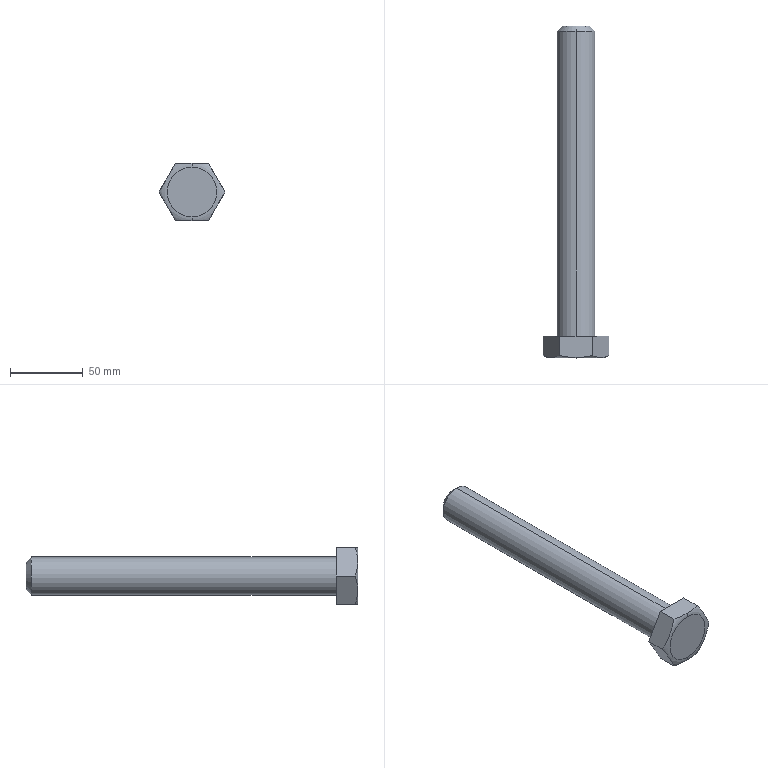Part | SolidWorks | features Chamfer 1, Extrusion 1, ICE 1, RevCut 1, Scale 1 | 1 solid | 15 faces | box 45.466 x 228.75 x 39.375 mm | volume 135169 mm3 | plane 9 | torus 2 | cone 2 | cylinder 2 | commonest cylinder face diameters 26.25 x2
STEP:
#1=CARTESIAN_POINT('',(11.367,-46.908,19.687));
#2=VERTEX_POINT('',#1);
#3=CARTESIAN_POINT('',(0.,-48.421,19.687));
#4=VERTEX_POINT('',#3);
#5=CARTESIAN_POINT('',(11.367,-46.908,19.687));
#6=CARTESIAN_POINT('',(10.465,-47.246,19.687));
#7=CARTESIAN_POINT('',(9.542,-47.5,19.687));
#8=CARTESIAN_POINT('',(7.671,-47.896,19.687));
#9=CARTESIAN_POINT('',(6.72,-48.038,19.687));
#10=CARTESIAN_POINT('',(4.805,-48.248,19.687));
#11=CARTESIAN_POINT('',(3.846,-48.315,19.687));
#12=CARTESIAN_POINT('',(1.925,-48.402,19.687));
#13=CARTESIAN_POINT('',(0.9641,-48.421,19.687));
#14=CARTESIAN_POINT('',(0.,-48.421,19.687));
#15=B_SPLINE_CURVE_WITH_KNOTS('',3,(#5,#6,#7,#8,#9,#10,#11,#12,#13,#14),.UNSPECIFIED.,.F.,.F.,(4,2,2,2,4),(0.07618,0.07906,0.08194,0.08482,0.08769),.UNSPECIFIED.);
#16=EDGE_CURVE('',#2,#4,#15,.T.);
#17=ORIENTED_EDGE('',*,*,#16,.T.);
#18=CARTESIAN_POINT('',(0.,-48.783,17.108));
#19=VERTEX_POINT('',#18);
#20=CARTESIAN_POINT('',(0.,-39.408,17.108));
#21=DIRECTION('',(1.,0.,0.));
#22=DIRECTION('',(0.,0.,-1.));
#23=AXIS2_PLACEMENT_3D('',#20,#21,#22);
#24=CIRCLE('',#23,9.375);
#25=EDGE_CURVE('',#4,#19,#24,.T.);
#26=ORIENTED_EDGE('',*,*,#25,.T.);
#27=CARTESIAN_POINT('',(0.,-48.783,-17.108));
#28=VERTEX_POINT('',#27);
#29=CARTESIAN_POINT('',(0.,-48.783,0.));
#30=DIRECTION('',(0.,-1.,0.));
#31=DIRECTION('',(0.,0.,-1.));
#32=AXIS2_PLACEMENT_3D('',#29,#30,#31);
#33=CIRCLE('',#32,17.108);
#34=EDGE_CURVE('',#28,#19,#33,.T.);
#35=ORIENTED_EDGE('',*,*,#34,.F.);
#36=CARTESIAN_POINT('',(0.,-48.421,-19.688));
#37=VERTEX_POINT('',#36);
#38=CARTESIAN_POINT('',(0.,-39.408,-17.108));
#39=DIRECTION('',(-1.,0.,0.));
#40=DIRECTION('',(0.,0.,1.));
#41=AXIS2_PLACEMENT_3D('',#38,#39,#40);
#42=CIRCLE('',#41,9.375);
#43=EDGE_CURVE('',#37,#28,#42,.T.);
#44=ORIENTED_EDGE('',*,*,#43,.F.);
#45=CARTESIAN_POINT('',(11.367,-46.908,-19.688));
#46=VERTEX_POINT('',#45);
#47=CARTESIAN_POINT('',(0.,-48.421,-19.688));
#48=CARTESIAN_POINT('',(0.9617,-48.421,-19.688));
#49=CARTESIAN_POINT('',(1.922,-48.402,-19.688));
#50=CARTESIAN_POINT('',(3.837,-48.315,-19.688));
#51=CARTESIAN_POINT('',(4.792,-48.248,-19.688));
#52=CARTESIAN_POINT('',(6.695,-48.041,-19.688));
#53=CARTESIAN_POINT('',(7.644,-47.901,-19.688));
#54=CARTESIAN_POINT('',(9.058,-47.603,-19.688));
#55=CARTESIAN_POINT('',(9.529,-47.488,-19.688));
#56=CARTESIAN_POINT('',(10.458,-47.226,-19.688));
#57=CARTESIAN_POINT('',(10.916,-47.077,-19.688));
#58=CARTESIAN_POINT('',(11.367,-46.908,-19.688));
#59=B_SPLINE_CURVE_WITH_KNOTS('',3,(#47,#48,#49,#50,#51,#52,#53,#54,#55,#56,#57,#58),.UNSPECIFIED.,.F.,.F.,(4,2,2,2,2,4),(0.,0.002872,0.005744,0.008616,0.01005,0.01149),.UNSPECIFIED.);
#60=EDGE_CURVE('',#37,#46,#59,.T.);
#61=ORIENTED_EDGE('',*,*,#60,.T.);
#62=CARTESIAN_POINT('',(22.733,-46.908,0.));
#63=VERTEX_POINT('',#62);
#64=CARTESIAN_POINT('',(11.367,-46.908,-19.688));
#65=CARTESIAN_POINT('',(11.821,-47.249,-18.901));
#66=CARTESIAN_POINT('',(12.283,-47.502,-18.1));
#67=CARTESIAN_POINT('',(13.219,-47.897,-16.479));
#68=CARTESIAN_POINT('',(13.693,-48.038,-15.659));
#69=CARTESIAN_POINT('',(14.646,-48.247,-14.007));
#70=CARTESIAN_POINT('',(15.128,-48.315,-13.173));
#71=CARTESIAN_POINT('',(16.087,-48.402,-11.511));
#72=CARTESIAN_POINT('',(16.567,-48.421,-10.681));
#73=CARTESIAN_POINT('',(17.524,-48.421,-9.022));
#74=CARTESIAN_POINT('',(18.003,-48.402,-8.193));
#75=CARTESIAN_POINT('',(18.959,-48.317,-6.537));
#76=CARTESIAN_POINT('',(19.437,-48.25,-5.709));
#77=CARTESIAN_POINT('',(20.152,-48.095,-4.47));
#78=CARTESIAN_POINT('',(20.391,-48.033,-4.057));
#79=CARTESIAN_POINT('',(20.867,-47.887,-3.233));
#80=CARTESIAN_POINT('',(21.105,-47.802,-2.82));
#81=CARTESIAN_POINT('',(21.814,-47.504,-1.591));
#82=CARTESIAN_POINT('',(22.28,-47.248,-0.7857));
#83=CARTESIAN_POINT('',(22.733,-46.908,0.));
#84=B_SPLINE_CURVE_WITH_KNOTS('',3,(#64,#65,#66,#67,#68,#69,#70,#71,#72,#73,#74,#75,#76,#77,#78,#79,#80,#81,#82,#83),.UNSPECIFIED.,.F.,.F.,(4,2,2,2,2,2,2,2,2,4),(0.000000456,0.00287,0.005739,0.008608,0.01148,0.01435,0.01722,0.01865,0.02008,0.02295),.UNSPECIFIED.);
#85=EDGE_CURVE('',#46,#63,#84,.T.);
#86=ORIENTED_EDGE('',*,*,#85,.T.);
#87=CARTESIAN_POINT('',(22.733,-46.908,0.));
#88=CARTESIAN_POINT('',(22.279,-47.249,0.7866));
#89=CARTESIAN_POINT('',(21.816,-47.502,1.588));
#90=CARTESIAN_POINT('',(20.881,-47.897,3.209));
#91=CARTESIAN_POINT('',(20.407,-48.038,4.029));
#92=CARTESIAN_POINT('',(19.453,-48.247,5.681));
#93=CARTESIAN_POINT('',(18.972,-48.315,6.514));
#94=CARTESIAN_POINT('',(18.013,-48.402,8.176));
#95=CARTESIAN_POINT('',(17.533,-48.421,9.007));
#96=CARTESIAN_POINT('',(16.575,-48.421,10.666));
#97=CARTESIAN_POINT('',(16.097,-48.402,11.495));
#98=CARTESIAN_POINT('',(15.14,-48.317,13.151));
#99=CARTESIAN_POINT('',(14.663,-48.25,13.978));
#100=CARTESIAN_POINT('',(13.947,-48.095,15.217));
#101=CARTESIAN_POINT('',(13.709,-48.033,15.63));
#102=CARTESIAN_POINT('',(13.233,-47.887,16.455));
#103=CARTESIAN_POINT('',(12.995,-47.802,16.868));
#104=CARTESIAN_POINT('',(12.285,-47.504,18.096));
#105=CARTESIAN_POINT('',(11.82,-47.248,18.902));
#106=CARTESIAN_POINT('',(11.367,-46.908,19.687));
#107=B_SPLINE_CURVE_WITH_KNOTS('',3,(#87,#88,#89,#90,#91,#92,#93,#94,#95,#96,#97,#98,#99,#100,#101,#102,#103,#104,#105,#106),.UNSPECIFIED.,.F.,.F.,(4,2,2,2,2,2,2,2,2,4),(0.000000456,0.00287,0.005739,0.008608,0.01148,0.01435,0.01722,0.01865,0.02008,0.02295),.UNSPECIFIED.);
#108=EDGE_CURVE('',#63,#2,#107,.T.);
#109=ORIENTED_EDGE('',*,*,#108,.T.);
#110=EDGE_LOOP('',(#17,#26,#35,#44,#61,#86,#109));
#111=FACE_OUTER_BOUND('',#110,.T.);
#112=CARTESIAN_POINT('',(0.,-39.408,0.));
#113=DIRECTION('',(0.,-1.,0.));
#114=DIRECTION('',(0.,0.,-1.));
#115=AXIS2_PLACEMENT_3D('',#112,#113,#114);
#116=TOROIDAL_SURFACE('',#115,17.108,9.375);
#117=ADVANCED_FACE('',(#111),#116,.T.);
#118=CARTESIAN_POINT('',(0.,179.967,9.375));
#119=VERTEX_POINT('',#118);
#120=CARTESIAN_POINT('',(0.,179.967,-9.375));
#121=VERTEX_POINT('',#120);
#122=CARTESIAN_POINT('',(0.,179.967,0.));
#123=DIRECTION('',(0.,1.,0.));
#124=DIRECTION('',(0.,0.,1.));
#125=AXIS2_PLACEMENT_3D('',#122,#123,#124);
#126=CIRCLE('',#125,9.375);
#127=EDGE_CURVE('',#119,#121,#126,.T.);
#128=ORIENTED_EDGE('',*,*,#127,.F.);
#129=CARTESIAN_POINT('',(0.,176.217,13.125));
#130=VERTEX_POINT('',#129);
#131=CARTESIAN_POINT('',(0.,179.967,9.375));
#132=DIRECTION('',(0.,-0.7071,0.7071));
#133=VECTOR('',#132,1000.);
#134=LINE('',#131,#133);
#135=EDGE_CURVE('',#119,#130,#134,.T.);
#136=ORIENTED_EDGE('',*,*,#135,.T.);
#137=CARTESIAN_POINT('',(0.,176.217,-13.125));
#138=VERTEX_POINT('',#137);
#139=CARTESIAN_POINT('',(0.,176.217,0.));
#140=DIRECTION('',(0.,-1.,0.));
#141=DIRECTION('',(0.,0.,1.));
#142=AXIS2_PLACEMENT_3D('',#139,#140,#141);
#143=CIRCLE('',#142,13.125);
#144=EDGE_CURVE('',#138,#130,#143,.T.);
#145=ORIENTED_EDGE('',*,*,#144,.F.);
#146=CARTESIAN_POINT('',(0.,179.967,-9.375));
#147=DIRECTION('',(0.,-0.7071,-0.7071));
#148=VECTOR('',#147,1000.);
#149=LINE('',#146,#148);
#150=EDGE_CURVE('',#121,#138,#149,.T.);
#151=ORIENTED_EDGE('',*,*,#150,.F.);
#152=EDGE_LOOP('',(#128,#136,#145,#151));
#153=FACE_OUTER_BOUND('',#152,.T.);
#154=CARTESIAN_POINT('',(0.,179.967,0.));
#155=DIRECTION('',(0.,-1.,0.));
#156=DIRECTION('',(0.,0.,-1.));
#157=AXIS2_PLACEMENT_3D('',#154,#155,#156);
#158=CONICAL_SURFACE('',#157,9.375,0.7854);
#159=ADVANCED_FACE('',(#153),#158,.T.);
#160=ORIENTED_EDGE('',*,*,#144,.T.);
#161=CARTESIAN_POINT('',(0.,-33.783,13.125));
#162=VERTEX_POINT('',#161);
#163=CARTESIAN_POINT('',(0.,179.967,13.125));
#164=DIRECTION('',(0.,-1.,0.));
#165=VECTOR('',#164,1000.);
#166=LINE('',#163,#165);
#167=EDGE_CURVE('',#130,#162,#166,.T.);
#168=ORIENTED_EDGE('',*,*,#167,.T.);
#169=CARTESIAN_POINT('',(0.,-33.783,-13.125));
#170=VERTEX_POINT('',#169);
#171=CARTESIAN_POINT('',(0.,-33.783,0.));
#172=DIRECTION('',(0.,1.,0.));
#173=DIRECTION('',(0.,0.,1.));
#174=AXIS2_PLACEMENT_3D('',#171,#172,#173);
#175=CIRCLE('',#174,13.125);
#176=EDGE_CURVE('',#162,#170,#175,.T.);
#177=ORIENTED_EDGE('',*,*,#176,.T.);
#178=CARTESIAN_POINT('',(0.,179.967,-13.125));
#179=DIRECTION('',(0.,-1.,0.));
#180=VECTOR('',#179,1000.);
#181=LINE('',#178,#180);
#182=EDGE_CURVE('',#138,#170,#181,.T.);
#183=ORIENTED_EDGE('',*,*,#182,.F.);
#184=EDGE_LOOP('',(#160,#168,#177,#183));
#185=FACE_OUTER_BOUND('',#184,.T.);
#186=CARTESIAN_POINT('',(0.,179.967,0.));
#187=DIRECTION('',(0.,-1.,0.));
#188=DIRECTION('',(0.,0.,-1.));
#189=AXIS2_PLACEMENT_3D('',#186,#187,#188);
#190=CYLINDRICAL_SURFACE('',#189,13.125);
#191=ADVANCED_FACE('',(#185),#190,.T.);
#192=ORIENTED_EDGE('',*,*,#108,.F.);
#193=CARTESIAN_POINT('',(22.733,-33.783,0.));
#194=VERTEX_POINT('',#193);
#195=CARTESIAN_POINT('',(22.733,-33.783,0.));
#196=DIRECTION('',(0.,-1.,0.));
#197=VECTOR('',#196,1000.);
#198=LINE('',#195,#197);
#199=EDGE_CURVE('',#194,#63,#198,.T.);
#200=ORIENTED_EDGE('',*,*,#199,.F.);
#201=CARTESIAN_POINT('',(11.367,-33.783,19.687));
#202=VERTEX_POINT('',#201);
#203=CARTESIAN_POINT('',(11.367,-33.783,19.687));
#204=DIRECTION('',(0.5,0.,-0.866));
#205=VECTOR('',#204,1000.);
#206=LINE('',#203,#205);
#207=EDGE_CURVE('',#202,#194,#206,.T.);
#208=ORIENTED_EDGE('',*,*,#207,.F.);
#209=CARTESIAN_POINT('',(11.367,-33.783,19.687));
#210=DIRECTION('',(0.,-1.,0.));
#211=VECTOR('',#210,1000.);
#212=LINE('',#209,#211);
#213=EDGE_CURVE('',#202,#2,#212,.T.);
#214=ORIENTED_EDGE('',*,*,#213,.T.);
#215=EDGE_LOOP('',(#192,#200,#208,#214));
#216=FACE_OUTER_BOUND('',#215,.T.);
#217=CARTESIAN_POINT('',(11.367,-33.783,19.687));
#218=DIRECTION('',(-0.866,0.,-0.5));
#219=DIRECTION('',(-0.5,0.,0.866));
#220=AXIS2_PLACEMENT_3D('',#217,#218,#219);
#221=PLANE('',#220);
#222=ADVANCED_FACE('',(#216),#221,.F.);
#223=ORIENTED_EDGE('',*,*,#85,.F.);
#224=CARTESIAN_POINT('',(11.367,-33.783,-19.688));
#225=VERTEX_POINT('',#224);
#226=CARTESIAN_POINT('',(11.367,-33.783,-19.688));
#227=DIRECTION('',(0.,-1.,0.));
#228=VECTOR('',#227,1000.);
#229=LINE('',#226,#228);
#230=EDGE_CURVE('',#225,#46,#229,.T.);
#231=ORIENTED_EDGE('',*,*,#230,.F.);
#232=CARTESIAN_POINT('',(22.733,-33.783,0.));
#233=DIRECTION('',(-0.5,0.,-0.866));
#234=VECTOR('',#233,1000.);
#235=LINE('',#232,#234);
#236=EDGE_CURVE('',#194,#225,#235,.T.);
#237=ORIENTED_EDGE('',*,*,#236,.F.);
#238=ORIENTED_EDGE('',*,*,#199,.T.);
#239=EDGE_LOOP('',(#223,#231,#237,#238));
#240=FACE_OUTER_BOUND('',#239,.T.);
#241=CARTESIAN_POINT('',(22.733,-33.783,0.));
#242=DIRECTION('',(-0.866,0.,0.5));
#243=DIRECTION('',(0.5,0.,0.866));
#244=AXIS2_PLACEMENT_3D('',#241,#242,#243);
#245=PLANE('',#244);
#246=ADVANCED_FACE('',(#240),#245,.F.);
#247=CARTESIAN_POINT('',(-11.367,-46.908,-19.688));
#248=VERTEX_POINT('',#247);
#249=CARTESIAN_POINT('',(-11.367,-46.908,-19.688));
#250=CARTESIAN_POINT('',(-10.465,-47.246,-19.688));
#251=CARTESIAN_POINT('',(-9.542,-47.5,-19.688));
#252=CARTESIAN_POINT('',(-7.671,-47.896,-19.687));
#253=CARTESIAN_POINT('',(-6.72,-48.038,-19.688));
#254=CARTESIAN_POINT('',(-4.805,-48.248,-19.688));
#255=CARTESIAN_POINT('',(-3.846,-48.315,-19.688));
#256=CARTESIAN_POINT('',(-1.925,-48.402,-19.688));
#257=CARTESIAN_POINT('',(-0.9641,-48.421,-19.688));
#258=CARTESIAN_POINT('',(0.,-48.421,-19.688));
#259=B_SPLINE_CURVE_WITH_KNOTS('',3,(#249,#250,#251,#252,#253,#254,#255,#256,#257,#258),.UNSPECIFIED.,.F.,.F.,(4,2,2,2,4),(0.07618,0.07906,0.08194,0.08482,0.08769),.UNSPECIFIED.);
#260=EDGE_CURVE('',#248,#37,#259,.T.);
#261=ORIENTED_EDGE('',*,*,#260,.F.);
#262=CARTESIAN_POINT('',(-11.367,-33.783,-19.688));
#263=VERTEX_POINT('',#262);
#264=CARTESIAN_POINT('',(-11.367,-33.783,-19.688));
#265=DIRECTION('',(0.,-1.,0.));
#266=VECTOR('',#265,1000.);
#267=LINE('',#264,#266);
#268=EDGE_CURVE('',#263,#248,#267,.T.);
#269=ORIENTED_EDGE('',*,*,#268,.F.);
#270=CARTESIAN_POINT('',(11.367,-33.783,-19.688));
#271=DIRECTION('',(-1.,0.,0.));
#272=VECTOR('',#271,1000.);
#273=LINE('',#270,#272);
#274=EDGE_CURVE('',#225,#263,#273,.T.);
#275=ORIENTED_EDGE('',*,*,#274,.F.);
#276=ORIENTED_EDGE('',*,*,#230,.T.);
#277=ORIENTED_EDGE('',*,*,#60,.F.);
#278=EDGE_LOOP('',(#261,#269,#275,#276,#277));
#279=FACE_OUTER_BOUND('',#278,.T.);
#280=CARTESIAN_POINT('',(11.367,-33.783,-19.688));
#281=DIRECTION('',(0.,0.,1.));
#282=DIRECTION('',(1.,0.,0.));
#283=AXIS2_PLACEMENT_3D('',#280,#281,#282);
#284=PLANE('',#283);
#285=ADVANCED_FACE('',(#279),#284,.F.);
#286=CARTESIAN_POINT('',(-22.733,-46.908,0.));
#287=VERTEX_POINT('',#286);
#288=CARTESIAN_POINT('',(-22.733,-46.908,0.));
#289=CARTESIAN_POINT('',(-22.279,-47.249,-0.7866));
#290=CARTESIAN_POINT('',(-21.816,-47.502,-1.588));
#291=CARTESIAN_POINT('',(-20.881,-47.897,-3.209));
#292=CARTESIAN_POINT('',(-20.407,-48.038,-4.029));
#293=CARTESIAN_POINT('',(-19.453,-48.247,-5.681));
#294=CARTESIAN_POINT('',(-18.972,-48.315,-6.514));
#295=CARTESIAN_POINT('',(-18.013,-48.402,-8.176));
#296=CARTESIAN_POINT('',(-17.533,-48.421,-9.007));
#297=CARTESIAN_POINT('',(-16.575,-48.421,-10.666));
#298=CARTESIAN_POINT('',(-16.097,-48.402,-11.495));
#299=CARTESIAN_POINT('',(-15.14,-48.317,-13.151));
#300=CARTESIAN_POINT('',(-14.663,-48.25,-13.978));
#301=CARTESIAN_POINT('',(-13.947,-48.095,-15.217));
#302=CARTESIAN_POINT('',(-13.709,-48.033,-15.63));
#303=CARTESIAN_POINT('',(-13.233,-47.887,-16.455));
#304=CARTESIAN_POINT('',(-12.995,-47.802,-16.868));
#305=CARTESIAN_POINT('',(-12.285,-47.504,-18.096));
#306=CARTESIAN_POINT('',(-11.82,-47.248,-18.902));
#307=CARTESIAN_POINT('',(-11.367,-46.908,-19.688));
#308=B_SPLINE_CURVE_WITH_KNOTS('',3,(#288,#289,#290,#291,#292,#293,#294,#295,#296,#297,#298,#299,#300,#301,#302,#303,#304,#305,#306,#307),.UNSPECIFIED.,.F.,.F.,(4,2,2,2,2,2,2,2,2,4),(0.000000456,0.00287,0.005739,0.008608,0.01148,0.01435,0.01722,0.01865,0.02008,0.02295),.UNSPECIFIED.);
#309=EDGE_CURVE('',#287,#248,#308,.T.);
#310=ORIENTED_EDGE('',*,*,#309,.F.);
#311=CARTESIAN_POINT('',(-22.733,-33.783,0.));
#312=VERTEX_POINT('',#311);
#313=CARTESIAN_POINT('',(-22.733,-33.783,0.));
#314=DIRECTION('',(0.,-1.,0.));
#315=VECTOR('',#314,1000.);
#316=LINE('',#313,#315);
#317=EDGE_CURVE('',#312,#287,#316,.T.);
#318=ORIENTED_EDGE('',*,*,#317,.F.);
#319=CARTESIAN_POINT('',(-11.367,-33.783,-19.688));
#320=DIRECTION('',(-0.5,0.,0.866));
#321=VECTOR('',#320,1000.);
#322=LINE('',#319,#321);
#323=EDGE_CURVE('',#263,#312,#322,.T.);
#324=ORIENTED_EDGE('',*,*,#323,.F.);
#325=ORIENTED_EDGE('',*,*,#268,.T.);
#326=EDGE_LOOP('',(#310,#318,#324,#325));
#327=FACE_OUTER_BOUND('',#326,.T.);
#328=CARTESIAN_POINT('',(-11.367,-33.783,-19.688));
#329=DIRECTION('',(0.866,0.,0.5));
#330=DIRECTION('',(0.5,0.,-0.866));
#331=AXIS2_PLACEMENT_3D('',#328,#329,#330);
#332=PLANE('',#331);
#333=ADVANCED_FACE('',(#327),#332,.F.);
#334=CARTESIAN_POINT('',(-11.367,-46.908,19.687));
#335=VERTEX_POINT('',#334);
#336=CARTESIAN_POINT('',(-11.367,-46.908,19.687));
#337=CARTESIAN_POINT('',(-11.821,-47.249,18.901));
#338=CARTESIAN_POINT('',(-12.283,-47.502,18.1));
#339=CARTESIAN_POINT('',(-13.219,-47.897,16.479));
#340=CARTESIAN_POINT('',(-13.693,-48.038,15.659));
#341=CARTESIAN_POINT('',(-14.646,-48.247,14.007));
#342=CARTESIAN_POINT('',(-15.128,-48.315,13.173));
#343=CARTESIAN_POINT('',(-16.087,-48.402,11.511));
#344=CARTESIAN_POINT('',(-16.567,-48.421,10.681));
#345=CARTESIAN_POINT('',(-17.524,-48.421,9.022));
#346=CARTESIAN_POINT('',(-18.003,-48.402,8.193));
#347=CARTESIAN_POINT('',(-18.959,-48.317,6.537));
#348=CARTESIAN_POINT('',(-19.437,-48.25,5.709));
#349=CARTESIAN_POINT('',(-20.152,-48.095,4.47));
#350=CARTESIAN_POINT('',(-20.391,-48.033,4.057));
#351=CARTESIAN_POINT('',(-20.867,-47.887,3.233));
#352=CARTESIAN_POINT('',(-21.105,-47.802,2.82));
#353=CARTESIAN_POINT('',(-21.814,-47.504,1.591));
#354=CARTESIAN_POINT('',(-22.28,-47.248,0.7857));
#355=CARTESIAN_POINT('',(-22.733,-46.908,0.));
#356=B_SPLINE_CURVE_WITH_KNOTS('',3,(#336,#337,#338,#339,#340,#341,#342,#343,#344,#345,#346,#347,#348,#349,#350,#351,#352,#353,#354,#355),.UNSPECIFIED.,.F.,.F.,(4,2,2,2,2,2,2,2,2,4),(0.000000456,0.00287,0.005739,0.008608,0.01148,0.01435,0.01722,0.01865,0.02008,0.02295),.UNSPECIFIED.);
#357=EDGE_CURVE('',#335,#287,#356,.T.);
#358=ORIENTED_EDGE('',*,*,#357,.F.);
#359=CARTESIAN_POINT('',(-11.367,-33.783,19.687));
#360=VERTEX_POINT('',#359);
#361=CARTESIAN_POINT('',(-11.367,-33.783,19.687));
#362=DIRECTION('',(0.,-1.,0.));
#363=VECTOR('',#362,1000.);
#364=LINE('',#361,#363);
#365=EDGE_CURVE('',#360,#335,#364,.T.);
#366=ORIENTED_EDGE('',*,*,#365,.F.);
#367=CARTESIAN_POINT('',(-22.733,-33.783,0.));
#368=DIRECTION('',(0.5,0.,0.866));
#369=VECTOR('',#368,1000.);
#370=LINE('',#367,#369);
#371=EDGE_CURVE('',#312,#360,#370,.T.);
#372=ORIENTED_EDGE('',*,*,#371,.F.);
#373=ORIENTED_EDGE('',*,*,#317,.T.);
#374=EDGE_LOOP('',(#358,#366,#372,#373));
#375=FACE_OUTER_BOUND('',#374,.T.);
#376=CARTESIAN_POINT('',(-22.733,-33.783,0.));
#377=DIRECTION('',(0.866,0.,-0.5));
#378=DIRECTION('',(-0.5,0.,-0.866));
#379=AXIS2_PLACEMENT_3D('',#376,#377,#378);
#380=PLANE('',#379);
#381=ADVANCED_FACE('',(#375),#380,.F.);
#382=ORIENTED_EDGE('',*,*,#16,.F.);
#383=ORIENTED_EDGE('',*,*,#213,.F.);
#384=CARTESIAN_POINT('',(-11.367,-33.783,19.687));
#385=DIRECTION('',(1.,0.,0.));
#386=VECTOR('',#385,1000.);
#387=LINE('',#384,#386);
#388=EDGE_CURVE('',#360,#202,#387,.T.);
#389=ORIENTED_EDGE('',*,*,#388,.F.);
#390=ORIENTED_EDGE('',*,*,#365,.T.);
#391=CARTESIAN_POINT('',(0.,-48.421,19.687));
#392=CARTESIAN_POINT('',(-0.9617,-48.421,19.687));
#393=CARTESIAN_POINT('',(-1.922,-48.402,19.687));
#394=CARTESIAN_POINT('',(-3.837,-48.315,19.687));
#395=CARTESIAN_POINT('',(-4.792,-48.248,19.687));
#396=CARTESIAN_POINT('',(-6.695,-48.041,19.687));
#397=CARTESIAN_POINT('',(-7.644,-47.901,19.687));
#398=CARTESIAN_POINT('',(-9.058,-47.603,19.687));
#399=CARTESIAN_POINT('',(-9.529,-47.488,19.687));
#400=CARTESIAN_POINT('',(-10.458,-47.226,19.687));
#401=CARTESIAN_POINT('',(-10.916,-47.077,19.687));
#402=CARTESIAN_POINT('',(-11.367,-46.908,19.687));
#403=B_SPLINE_CURVE_WITH_KNOTS('',3,(#391,#392,#393,#394,#395,#396,#397,#398,#399,#400,#401,#402),.UNSPECIFIED.,.F.,.F.,(4,2,2,2,2,4),(0.,0.002872,0.005744,0.008616,0.01005,0.01149),.UNSPECIFIED.);
#404=EDGE_CURVE('',#4,#335,#403,.T.);
#405=ORIENTED_EDGE('',*,*,#404,.F.);
#406=EDGE_LOOP('',(#382,#383,#389,#390,#405));
#407=FACE_OUTER_BOUND('',#406,.T.);
#408=CARTESIAN_POINT('',(-11.367,-33.783,19.687));
#409=DIRECTION('',(0.,0.,-1.));
#410=DIRECTION('',(-1.,0.,0.));
#411=AXIS2_PLACEMENT_3D('',#408,#409,#410);
#412=PLANE('',#411);
#413=ADVANCED_FACE('',(#407),#412,.F.);
#414=ORIENTED_EDGE('',*,*,#207,.T.);
#415=ORIENTED_EDGE('',*,*,#236,.T.);
#416=ORIENTED_EDGE('',*,*,#274,.T.);
#417=ORIENTED_EDGE('',*,*,#323,.T.);
#418=ORIENTED_EDGE('',*,*,#371,.T.);
#419=ORIENTED_EDGE('',*,*,#388,.T.);
#420=EDGE_LOOP('',(#414,#415,#416,#417,#418,#419));
#421=FACE_OUTER_BOUND('',#420,.T.);
#422=CARTESIAN_POINT('',(0.,-33.783,0.));
#423=DIRECTION('',(0.,1.,0.));
#424=DIRECTION('',(0.,0.,1.));
#425=AXIS2_PLACEMENT_3D('',#422,#423,#424);
#426=CIRCLE('',#425,13.125);
#427=EDGE_CURVE('',#170,#162,#426,.T.);
#428=ORIENTED_EDGE('',*,*,#427,.F.);
#429=ORIENTED_EDGE('',*,*,#176,.F.);
#430=EDGE_LOOP('',(#428,#429));
#431=FACE_BOUND('',#430,.T.);
#432=CARTESIAN_POINT('',(0.,-33.783,0.));
#433=DIRECTION('',(0.,1.,0.));
#434=DIRECTION('',(0.,0.,1.));
#435=AXIS2_PLACEMENT_3D('',#432,#433,#434);
#436=PLANE('',#435);
#437=ADVANCED_FACE('',(#421,#431),#436,.T.);
#438=ORIENTED_EDGE('',*,*,#167,.F.);
#439=CARTESIAN_POINT('',(0.,176.217,0.));
#440=DIRECTION('',(0.,-1.,0.));
#441=DIRECTION('',(0.,0.,1.));
#442=AXIS2_PLACEMENT_3D('',#439,#440,#441);
#443=CIRCLE('',#442,13.125);
#444=EDGE_CURVE('',#130,#138,#443,.T.);
#445=ORIENTED_EDGE('',*,*,#444,.T.);
#446=ORIENTED_EDGE('',*,*,#182,.T.);
#447=ORIENTED_EDGE('',*,*,#427,.T.);
#448=EDGE_LOOP('',(#438,#445,#446,#447));
#449=FACE_OUTER_BOUND('',#448,.T.);
#450=CARTESIAN_POINT('',(0.,179.967,0.));
#451=DIRECTION('',(0.,-1.,0.));
#452=DIRECTION('',(0.,0.,-1.));
#453=AXIS2_PLACEMENT_3D('',#450,#451,#452);
#454=CYLINDRICAL_SURFACE('',#453,13.125);
#455=ADVANCED_FACE('',(#449),#454,.T.);
#456=CARTESIAN_POINT('',(0.,179.967,0.));
#457=DIRECTION('',(0.,1.,0.));
#458=DIRECTION('',(0.,0.,1.));
#459=AXIS2_PLACEMENT_3D('',#456,#457,#458);
#460=CIRCLE('',#459,9.375);
#461=EDGE_CURVE('',#121,#119,#460,.T.);
#462=ORIENTED_EDGE('',*,*,#461,.T.);
#463=ORIENTED_EDGE('',*,*,#127,.T.);
#464=EDGE_LOOP('',(#462,#463));
#465=FACE_OUTER_BOUND('',#464,.T.);
#466=CARTESIAN_POINT('',(0.,179.967,0.));
#467=DIRECTION('',(0.,1.,0.));
#468=DIRECTION('',(0.,0.,1.));
#469=AXIS2_PLACEMENT_3D('',#466,#467,#468);
#470=PLANE('',#469);
#471=ADVANCED_FACE('',(#465),#470,.T.);
#472=ORIENTED_EDGE('',*,*,#135,.F.);
#473=ORIENTED_EDGE('',*,*,#461,.F.);
#474=ORIENTED_EDGE('',*,*,#150,.T.);
#475=ORIENTED_EDGE('',*,*,#444,.F.);
#476=EDGE_LOOP('',(#472,#473,#474,#475));
#477=FACE_OUTER_BOUND('',#476,.T.);
#478=CARTESIAN_POINT('',(0.,179.967,0.));
#479=DIRECTION('',(0.,-1.,0.));
#480=DIRECTION('',(0.,0.,-1.));
#481=AXIS2_PLACEMENT_3D('',#478,#479,#480);
#482=CONICAL_SURFACE('',#481,9.375,0.7854);
#483=ADVANCED_FACE('',(#477),#482,.T.);
#484=ORIENTED_EDGE('',*,*,#25,.F.);
#485=ORIENTED_EDGE('',*,*,#404,.T.);
#486=ORIENTED_EDGE('',*,*,#357,.T.);
#487=ORIENTED_EDGE('',*,*,#309,.T.);
#488=ORIENTED_EDGE('',*,*,#260,.T.);
#489=ORIENTED_EDGE('',*,*,#43,.T.);
#490=CARTESIAN_POINT('',(0.,-48.783,0.));
#491=DIRECTION('',(0.,-1.,0.));
#492=DIRECTION('',(0.,0.,-1.));
#493=AXIS2_PLACEMENT_3D('',#490,#491,#492);
#494=CIRCLE('',#493,17.108);
#495=EDGE_CURVE('',#19,#28,#494,.T.);
#496=ORIENTED_EDGE('',*,*,#495,.F.);
#497=EDGE_LOOP('',(#484,#485,#486,#487,#488,#489,#496));
#498=FACE_OUTER_BOUND('',#497,.T.);
#499=CARTESIAN_POINT('',(0.,-39.408,0.));
#500=DIRECTION('',(0.,-1.,0.));
#501=DIRECTION('',(0.,0.,-1.));
#502=AXIS2_PLACEMENT_3D('',#499,#500,#501);
#503=TOROIDAL_SURFACE('',#502,17.108,9.375);
#504=ADVANCED_FACE('',(#498),#503,.T.);
#505=ORIENTED_EDGE('',*,*,#34,.T.);
#506=ORIENTED_EDGE('',*,*,#495,.T.);
#507=EDGE_LOOP('',(#505,#506));
#508=FACE_OUTER_BOUND('',#507,.T.);
#509=CARTESIAN_POINT('',(0.,-48.783,0.));
#510=DIRECTION('',(0.,1.,0.));
#511=DIRECTION('',(0.,0.,1.));
#512=AXIS2_PLACEMENT_3D('',#509,#510,#511);
#513=PLANE('',#512);
#514=ADVANCED_FACE('',(#508),#513,.F.);
#515=CLOSED_SHELL('',(#117,#159,#191,#222,#246,#285,#333,#381,#413,#437,#455,#471,#483,#504,#514));
#516=MANIFOLD_SOLID_BREP('',#515);
#517=CARTESIAN_POINT('',(0.,0.,0.));
#518=DIRECTION('',(0.,0.,1.));
#519=DIRECTION('',(1.,0.,0.));
#520=AXIS2_PLACEMENT_3D('',#517,#518,#519);
#521=(LENGTH_UNIT()NAMED_UNIT(*)SI_UNIT(.MILLI.,.METRE.));
#522=UNCERTAINTY_MEASURE_WITH_UNIT(LENGTH_MEASURE(0.00001),#521,'','');
#523=(NAMED_UNIT(*)PLANE_ANGLE_UNIT()SI_UNIT($,.RADIAN.));
#524=(NAMED_UNIT(*)SI_UNIT($,.STERADIAN.)SOLID_ANGLE_UNIT());
#525=(GEOMETRIC_REPRESENTATION_CONTEXT(3)GLOBAL_UNCERTAINTY_ASSIGNED_CONTEXT((#522))GLOBAL_UNIT_ASSIGNED_CONTEXT((#521,#523,#524))REPRESENTATION_CONTEXT('',''));
#526=ADVANCED_BREP_SHAPE_REPRESENTATION('',(#516,#520),#525);